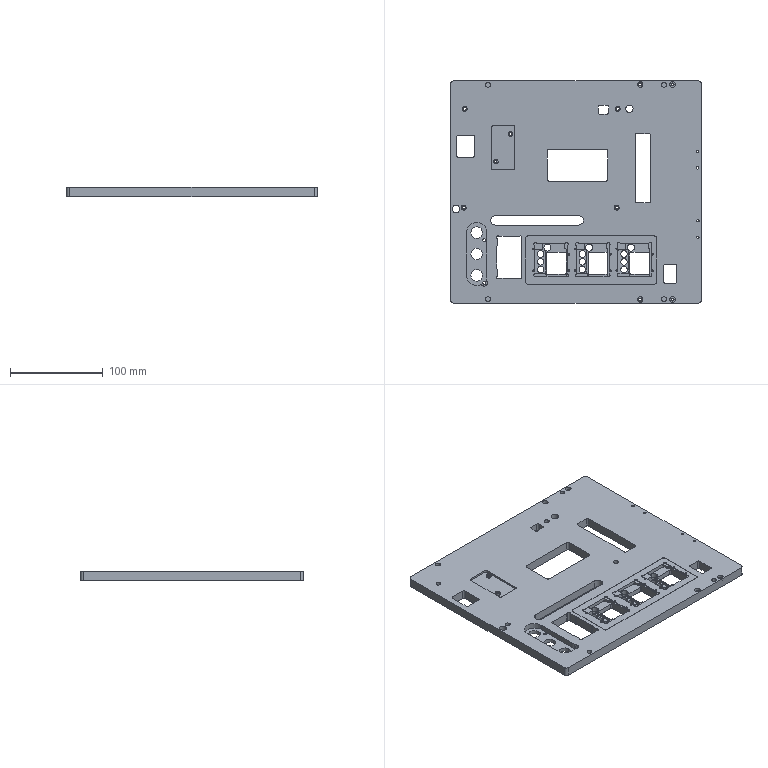Part | 1 solid | 606 faces | box 270 x 240 x 10 mm | volume 538627 mm3 | plane 271 | cylinder 260 | cone 39 | spline 36 | commonest cylinder face diameters 3.5 x52 2 x51 1.6 x24 3.2 x20 7 x20 5.25 x16